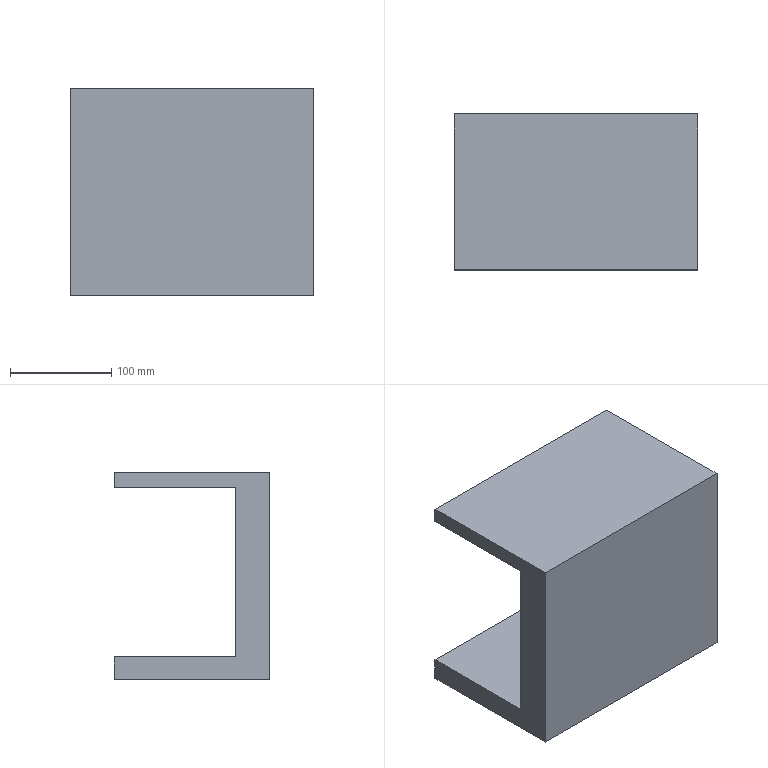Part | STEP file | Part 16^超升波生产线-2 | 1 solid | 10 faces | box 240.448 x 154.13 x 205 mm | volume 2766598 mm3 | plane 10
STEP:
#1=CARTESIAN_POINT('',(122.789,197.065,205.));
#2=VERTEX_POINT('',#1);
#3=CARTESIAN_POINT('',(122.789,197.065,190.));
#4=VERTEX_POINT('',#3);
#5=CARTESIAN_POINT('',(122.789,197.065,205.));
#6=DIRECTION('',(0.,0.,-1.));
#7=VECTOR('',#6,1000.);
#8=LINE('',#5,#7);
#9=EDGE_CURVE('',#2,#4,#8,.T.);
#10=ORIENTED_EDGE('',*,*,#9,.T.);
#11=CARTESIAN_POINT('',(-117.659,197.065,190.));
#12=VERTEX_POINT('',#11);
#13=CARTESIAN_POINT('',(122.789,197.065,190.));
#14=DIRECTION('',(-1.,0.,0.));
#15=VECTOR('',#14,1000.);
#16=LINE('',#13,#15);
#17=EDGE_CURVE('',#4,#12,#16,.T.);
#18=ORIENTED_EDGE('',*,*,#17,.T.);
#19=CARTESIAN_POINT('',(-117.659,197.065,205.));
#20=VERTEX_POINT('',#19);
#21=CARTESIAN_POINT('',(-117.659,197.065,205.));
#22=DIRECTION('',(0.,0.,-1.));
#23=VECTOR('',#22,1000.);
#24=LINE('',#21,#23);
#25=EDGE_CURVE('',#20,#12,#24,.T.);
#26=ORIENTED_EDGE('',*,*,#25,.F.);
#27=CARTESIAN_POINT('',(-117.659,197.065,205.));
#28=DIRECTION('',(-1.,0.,0.));
#29=VECTOR('',#28,1000.);
#30=LINE('',#27,#29);
#31=EDGE_CURVE('',#2,#20,#30,.T.);
#32=ORIENTED_EDGE('',*,*,#31,.F.);
#33=EDGE_LOOP('',(#10,#18,#26,#32));
#34=FACE_OUTER_BOUND('',#33,.T.);
#35=CARTESIAN_POINT('',(-117.659,197.065,205.));
#36=DIRECTION('',(0.,-1.,0.));
#37=DIRECTION('',(0.,0.,-1.));
#38=AXIS2_PLACEMENT_3D('',#35,#36,#37);
#39=PLANE('',#38);
#40=ADVANCED_FACE('',(#34),#39,.F.);
#41=CARTESIAN_POINT('',(122.789,77.034,22.622));
#42=VERTEX_POINT('',#41);
#43=CARTESIAN_POINT('',(122.789,77.034,190.));
#44=VERTEX_POINT('',#43);
#45=CARTESIAN_POINT('',(122.789,77.034,190.));
#46=DIRECTION('',(0.,0.,1.));
#47=VECTOR('',#46,1000.);
#48=LINE('',#45,#47);
#49=EDGE_CURVE('',#42,#44,#48,.T.);
#50=ORIENTED_EDGE('',*,*,#49,.T.);
#51=CARTESIAN_POINT('',(122.789,197.065,190.));
#52=DIRECTION('',(0.,1.,0.));
#53=VECTOR('',#52,1000.);
#54=LINE('',#51,#53);
#55=EDGE_CURVE('',#44,#4,#54,.T.);
#56=ORIENTED_EDGE('',*,*,#55,.T.);
#57=ORIENTED_EDGE('',*,*,#9,.F.);
#58=CARTESIAN_POINT('',(122.789,42.935,205.));
#59=VERTEX_POINT('',#58);
#60=CARTESIAN_POINT('',(122.789,42.935,205.));
#61=DIRECTION('',(0.,1.,0.));
#62=VECTOR('',#61,1000.);
#63=LINE('',#60,#62);
#64=EDGE_CURVE('',#59,#2,#63,.T.);
#65=ORIENTED_EDGE('',*,*,#64,.F.);
#66=CARTESIAN_POINT('',(122.789,42.935,0.));
#67=VERTEX_POINT('',#66);
#68=CARTESIAN_POINT('',(122.789,42.935,205.));
#69=DIRECTION('',(0.,0.,-1.));
#70=VECTOR('',#69,1000.);
#71=LINE('',#68,#70);
#72=EDGE_CURVE('',#59,#67,#71,.T.);
#73=ORIENTED_EDGE('',*,*,#72,.T.);
#74=CARTESIAN_POINT('',(122.789,197.065,0.));
#75=VERTEX_POINT('',#74);
#76=CARTESIAN_POINT('',(122.789,42.935,0.));
#77=DIRECTION('',(0.,1.,0.));
#78=VECTOR('',#77,1000.);
#79=LINE('',#76,#78);
#80=EDGE_CURVE('',#67,#75,#79,.T.);
#81=ORIENTED_EDGE('',*,*,#80,.T.);
#82=CARTESIAN_POINT('',(122.789,197.065,22.622));
#83=VERTEX_POINT('',#82);
#84=CARTESIAN_POINT('',(122.789,197.065,205.));
#85=DIRECTION('',(0.,0.,-1.));
#86=VECTOR('',#85,1000.);
#87=LINE('',#84,#86);
#88=EDGE_CURVE('',#83,#75,#87,.T.);
#89=ORIENTED_EDGE('',*,*,#88,.F.);
#90=CARTESIAN_POINT('',(122.789,197.065,22.622));
#91=DIRECTION('',(0.,-1.,0.));
#92=VECTOR('',#91,1000.);
#93=LINE('',#90,#92);
#94=EDGE_CURVE('',#83,#42,#93,.T.);
#95=ORIENTED_EDGE('',*,*,#94,.T.);
#96=EDGE_LOOP('',(#50,#56,#57,#65,#73,#81,#89,#95));
#97=FACE_OUTER_BOUND('',#96,.T.);
#98=CARTESIAN_POINT('',(122.789,42.935,205.));
#99=DIRECTION('',(-1.,0.,0.));
#100=DIRECTION('',(0.,0.,1.));
#101=AXIS2_PLACEMENT_3D('',#98,#99,#100);
#102=PLANE('',#101);
#103=ADVANCED_FACE('',(#97),#102,.F.);
#104=CARTESIAN_POINT('',(-117.659,197.065,22.622));
#105=VERTEX_POINT('',#104);
#106=CARTESIAN_POINT('',(-117.659,197.065,0.));
#107=VERTEX_POINT('',#106);
#108=CARTESIAN_POINT('',(-117.659,197.065,205.));
#109=DIRECTION('',(0.,0.,-1.));
#110=VECTOR('',#109,1000.);
#111=LINE('',#108,#110);
#112=EDGE_CURVE('',#105,#107,#111,.T.);
#113=ORIENTED_EDGE('',*,*,#112,.F.);
#114=CARTESIAN_POINT('',(122.789,197.065,22.622));
#115=DIRECTION('',(-1.,0.,0.));
#116=VECTOR('',#115,1000.);
#117=LINE('',#114,#116);
#118=EDGE_CURVE('',#83,#105,#117,.T.);
#119=ORIENTED_EDGE('',*,*,#118,.F.);
#120=ORIENTED_EDGE('',*,*,#88,.T.);
#121=CARTESIAN_POINT('',(-117.659,197.065,0.));
#122=DIRECTION('',(-1.,0.,0.));
#123=VECTOR('',#122,1000.);
#124=LINE('',#121,#123);
#125=EDGE_CURVE('',#75,#107,#124,.T.);
#126=ORIENTED_EDGE('',*,*,#125,.T.);
#127=EDGE_LOOP('',(#113,#119,#120,#126));
#128=FACE_OUTER_BOUND('',#127,.T.);
#129=CARTESIAN_POINT('',(-117.659,197.065,205.));
#130=DIRECTION('',(0.,-1.,0.));
#131=DIRECTION('',(0.,0.,-1.));
#132=AXIS2_PLACEMENT_3D('',#129,#130,#131);
#133=PLANE('',#132);
#134=ADVANCED_FACE('',(#128),#133,.F.);
#135=ORIENTED_EDGE('',*,*,#25,.T.);
#136=CARTESIAN_POINT('',(-117.659,77.034,190.));
#137=VERTEX_POINT('',#136);
#138=CARTESIAN_POINT('',(-117.659,197.065,190.));
#139=DIRECTION('',(0.,1.,0.));
#140=VECTOR('',#139,1000.);
#141=LINE('',#138,#140);
#142=EDGE_CURVE('',#137,#12,#141,.T.);
#143=ORIENTED_EDGE('',*,*,#142,.F.);
#144=CARTESIAN_POINT('',(-117.659,77.034,22.622));
#145=VERTEX_POINT('',#144);
#146=CARTESIAN_POINT('',(-117.659,77.034,190.));
#147=DIRECTION('',(0.,0.,1.));
#148=VECTOR('',#147,1000.);
#149=LINE('',#146,#148);
#150=EDGE_CURVE('',#145,#137,#149,.T.);
#151=ORIENTED_EDGE('',*,*,#150,.F.);
#152=CARTESIAN_POINT('',(-117.659,197.065,22.622));
#153=DIRECTION('',(0.,-1.,0.));
#154=VECTOR('',#153,1000.);
#155=LINE('',#152,#154);
#156=EDGE_CURVE('',#105,#145,#155,.T.);
#157=ORIENTED_EDGE('',*,*,#156,.F.);
#158=ORIENTED_EDGE('',*,*,#112,.T.);
#159=CARTESIAN_POINT('',(-117.659,42.935,0.));
#160=VERTEX_POINT('',#159);
#161=CARTESIAN_POINT('',(-117.659,42.935,0.));
#162=DIRECTION('',(0.,-1.,0.));
#163=VECTOR('',#162,1000.);
#164=LINE('',#161,#163);
#165=EDGE_CURVE('',#107,#160,#164,.T.);
#166=ORIENTED_EDGE('',*,*,#165,.T.);
#167=CARTESIAN_POINT('',(-117.659,42.935,205.));
#168=VERTEX_POINT('',#167);
#169=CARTESIAN_POINT('',(-117.659,42.935,205.));
#170=DIRECTION('',(0.,0.,-1.));
#171=VECTOR('',#170,1000.);
#172=LINE('',#169,#171);
#173=EDGE_CURVE('',#168,#160,#172,.T.);
#174=ORIENTED_EDGE('',*,*,#173,.F.);
#175=CARTESIAN_POINT('',(-117.659,42.935,205.));
#176=DIRECTION('',(0.,-1.,0.));
#177=VECTOR('',#176,1000.);
#178=LINE('',#175,#177);
#179=EDGE_CURVE('',#20,#168,#178,.T.);
#180=ORIENTED_EDGE('',*,*,#179,.F.);
#181=EDGE_LOOP('',(#135,#143,#151,#157,#158,#166,#174,#180));
#182=FACE_OUTER_BOUND('',#181,.T.);
#183=CARTESIAN_POINT('',(-117.659,42.935,205.));
#184=DIRECTION('',(1.,0.,0.));
#185=DIRECTION('',(0.,0.,-1.));
#186=AXIS2_PLACEMENT_3D('',#183,#184,#185);
#187=PLANE('',#186);
#188=ADVANCED_FACE('',(#182),#187,.F.);
#189=CARTESIAN_POINT('',(-117.659,42.935,0.));
#190=DIRECTION('',(1.,0.,0.));
#191=VECTOR('',#190,1000.);
#192=LINE('',#189,#191);
#193=EDGE_CURVE('',#160,#67,#192,.T.);
#194=ORIENTED_EDGE('',*,*,#193,.T.);
#195=ORIENTED_EDGE('',*,*,#72,.F.);
#196=CARTESIAN_POINT('',(-117.659,42.935,205.));
#197=DIRECTION('',(1.,0.,0.));
#198=VECTOR('',#197,1000.);
#199=LINE('',#196,#198);
#200=EDGE_CURVE('',#168,#59,#199,.T.);
#201=ORIENTED_EDGE('',*,*,#200,.F.);
#202=ORIENTED_EDGE('',*,*,#173,.T.);
#203=EDGE_LOOP('',(#194,#195,#201,#202));
#204=FACE_OUTER_BOUND('',#203,.T.);
#205=CARTESIAN_POINT('',(-117.659,42.935,205.));
#206=DIRECTION('',(0.,1.,0.));
#207=DIRECTION('',(0.,0.,1.));
#208=AXIS2_PLACEMENT_3D('',#205,#206,#207);
#209=PLANE('',#208);
#210=ADVANCED_FACE('',(#204),#209,.F.);
#211=ORIENTED_EDGE('',*,*,#64,.T.);
#212=ORIENTED_EDGE('',*,*,#31,.T.);
#213=ORIENTED_EDGE('',*,*,#179,.T.);
#214=ORIENTED_EDGE('',*,*,#200,.T.);
#215=EDGE_LOOP('',(#211,#212,#213,#214));
#216=FACE_OUTER_BOUND('',#215,.T.);
#217=CARTESIAN_POINT('',(122.789,197.065,205.));
#218=DIRECTION('',(0.,0.,-1.));
#219=DIRECTION('',(-1.,0.,0.));
#220=AXIS2_PLACEMENT_3D('',#217,#218,#219);
#221=PLANE('',#220);
#222=ADVANCED_FACE('',(#216),#221,.F.);
#223=ORIENTED_EDGE('',*,*,#80,.F.);
#224=ORIENTED_EDGE('',*,*,#193,.F.);
#225=ORIENTED_EDGE('',*,*,#165,.F.);
#226=ORIENTED_EDGE('',*,*,#125,.F.);
#227=EDGE_LOOP('',(#223,#224,#225,#226));
#228=FACE_OUTER_BOUND('',#227,.T.);
#229=CARTESIAN_POINT('',(122.789,197.065,0.));
#230=DIRECTION('',(0.,0.,-1.));
#231=DIRECTION('',(-1.,0.,0.));
#232=AXIS2_PLACEMENT_3D('',#229,#230,#231);
#233=PLANE('',#232);
#234=ADVANCED_FACE('',(#228),#233,.T.);
#235=ORIENTED_EDGE('',*,*,#142,.T.);
#236=ORIENTED_EDGE('',*,*,#17,.F.);
#237=ORIENTED_EDGE('',*,*,#55,.F.);
#238=CARTESIAN_POINT('',(122.789,77.034,190.));
#239=DIRECTION('',(-1.,0.,0.));
#240=VECTOR('',#239,1000.);
#241=LINE('',#238,#240);
#242=EDGE_CURVE('',#44,#137,#241,.T.);
#243=ORIENTED_EDGE('',*,*,#242,.T.);
#244=EDGE_LOOP('',(#235,#236,#237,#243));
#245=FACE_OUTER_BOUND('',#244,.T.);
#246=CARTESIAN_POINT('',(122.789,197.065,190.));
#247=DIRECTION('',(0.,0.,1.));
#248=DIRECTION('',(0.,-1.,0.));
#249=AXIS2_PLACEMENT_3D('',#246,#247,#248);
#250=PLANE('',#249);
#251=ADVANCED_FACE('',(#245),#250,.F.);
#252=ORIENTED_EDGE('',*,*,#150,.T.);
#253=ORIENTED_EDGE('',*,*,#242,.F.);
#254=ORIENTED_EDGE('',*,*,#49,.F.);
#255=CARTESIAN_POINT('',(122.789,77.034,22.622));
#256=DIRECTION('',(-1.,0.,0.));
#257=VECTOR('',#256,1000.);
#258=LINE('',#255,#257);
#259=EDGE_CURVE('',#42,#145,#258,.T.);
#260=ORIENTED_EDGE('',*,*,#259,.T.);
#261=EDGE_LOOP('',(#252,#253,#254,#260));
#262=FACE_OUTER_BOUND('',#261,.T.);
#263=CARTESIAN_POINT('',(122.789,77.034,190.));
#264=DIRECTION('',(0.,-1.,0.));
#265=DIRECTION('',(0.,0.,-1.));
#266=AXIS2_PLACEMENT_3D('',#263,#264,#265);
#267=PLANE('',#266);
#268=ADVANCED_FACE('',(#262),#267,.F.);
#269=ORIENTED_EDGE('',*,*,#156,.T.);
#270=ORIENTED_EDGE('',*,*,#259,.F.);
#271=ORIENTED_EDGE('',*,*,#94,.F.);
#272=ORIENTED_EDGE('',*,*,#118,.T.);
#273=EDGE_LOOP('',(#269,#270,#271,#272));
#274=FACE_OUTER_BOUND('',#273,.T.);
#275=CARTESIAN_POINT('',(122.789,197.065,22.622));
#276=DIRECTION('',(0.,0.,-1.));
#277=DIRECTION('',(-1.,0.,0.));
#278=AXIS2_PLACEMENT_3D('',#275,#276,#277);
#279=PLANE('',#278);
#280=ADVANCED_FACE('',(#274),#279,.F.);
#281=CLOSED_SHELL('',(#40,#103,#134,#188,#210,#222,#234,#251,#268,#280));
#282=MANIFOLD_SOLID_BREP('',#281);
#283=CARTESIAN_POINT('',(0.,0.,0.));
#284=DIRECTION('',(0.,0.,1.));
#285=DIRECTION('',(1.,0.,0.));
#286=AXIS2_PLACEMENT_3D('',#283,#284,#285);
#287=(LENGTH_UNIT()NAMED_UNIT(*)SI_UNIT(.MILLI.,.METRE.));
#288=UNCERTAINTY_MEASURE_WITH_UNIT(LENGTH_MEASURE(0.00001),#287,'','');
#289=(NAMED_UNIT(*)PLANE_ANGLE_UNIT()SI_UNIT($,.RADIAN.));
#290=(NAMED_UNIT(*)SI_UNIT($,.STERADIAN.)SOLID_ANGLE_UNIT());
#291=(GEOMETRIC_REPRESENTATION_CONTEXT(3)GLOBAL_UNCERTAINTY_ASSIGNED_CONTEXT((#288))GLOBAL_UNIT_ASSIGNED_CONTEXT((#287,#289,#290))REPRESENTATION_CONTEXT('',''));
#292=ADVANCED_BREP_SHAPE_REPRESENTATION('',(#282,#286),#291);